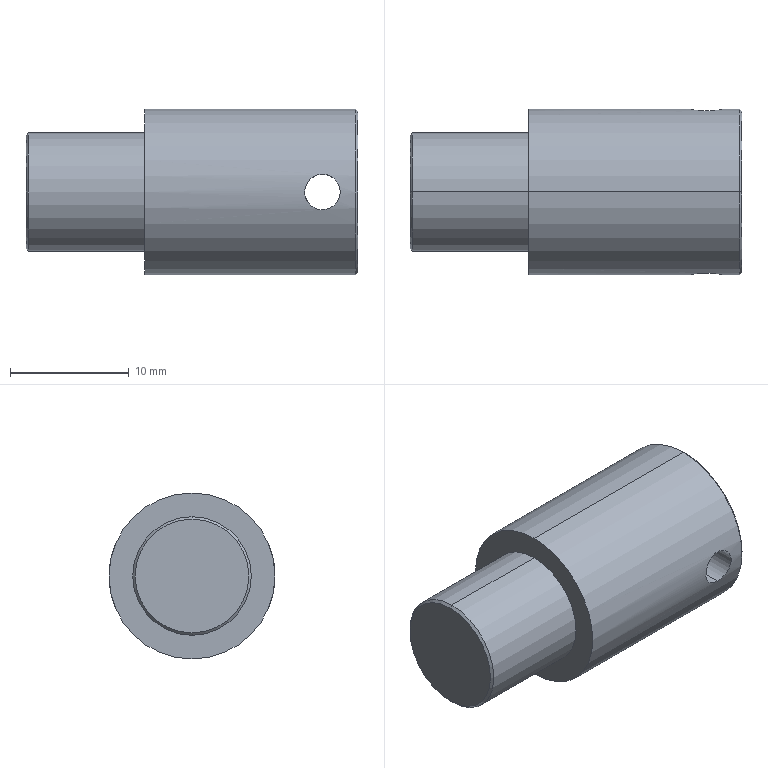Part | SolidWorks | features Chamfer 2, ICE 2, Revolution 1 | 1 solid | 13 faces | box 28 x 14 x 14 mm | volume 3456 mm3 | cylinder 6 | cone 4 | plane 3 | commonest cylinder face diameters 3 x2 10 x2 14 x2
STEP:
#1=CARTESIAN_POINT('',(28.,0.,-6.8));
#2=VERTEX_POINT('',#1);
#3=CARTESIAN_POINT('',(28.,0.,6.8));
#4=VERTEX_POINT('',#3);
#5=CARTESIAN_POINT('',(28.,0.,0.));
#6=DIRECTION('',(1.,0.,0.));
#7=DIRECTION('',(0.,0.,1.));
#8=AXIS2_PLACEMENT_3D('',#5,#6,#7);
#9=CIRCLE('',#8,6.8);
#10=EDGE_CURVE('',#2,#4,#9,.T.);
#11=ORIENTED_EDGE('',*,*,#10,.F.);
#12=CARTESIAN_POINT('',(27.8,0.,-7.));
#13=VERTEX_POINT('',#12);
#14=CARTESIAN_POINT('',(27.8,0.,-7.));
#15=DIRECTION('',(-0.7071,0.,-0.7071));
#16=VECTOR('',#15,1000.);
#17=LINE('',#14,#16);
#18=EDGE_CURVE('',#2,#13,#17,.T.);
#19=ORIENTED_EDGE('',*,*,#18,.T.);
#20=CARTESIAN_POINT('',(27.8,0.,7.));
#21=VERTEX_POINT('',#20);
#22=CARTESIAN_POINT('',(27.8,0.,0.));
#23=DIRECTION('',(-1.,0.,0.));
#24=DIRECTION('',(0.,0.,1.));
#25=AXIS2_PLACEMENT_3D('',#22,#23,#24);
#26=CIRCLE('',#25,7.);
#27=EDGE_CURVE('',#21,#13,#26,.T.);
#28=ORIENTED_EDGE('',*,*,#27,.F.);
#29=CARTESIAN_POINT('',(27.8,0.,7.));
#30=DIRECTION('',(-0.7071,0.,0.7071));
#31=VECTOR('',#30,1000.);
#32=LINE('',#29,#31);
#33=EDGE_CURVE('',#4,#21,#32,.T.);
#34=ORIENTED_EDGE('',*,*,#33,.F.);
#35=EDGE_LOOP('',(#11,#19,#28,#34));
#36=FACE_OUTER_BOUND('',#35,.T.);
#37=CARTESIAN_POINT('',(27.8,0.,0.));
#38=DIRECTION('',(-1.,0.,0.));
#39=DIRECTION('',(0.,0.,1.));
#40=AXIS2_PLACEMENT_3D('',#37,#38,#39);
#41=CONICAL_SURFACE('',#40,7.,0.7854);
#42=ADVANCED_FACE('',(#36),#41,.T.);
#43=CARTESIAN_POINT('',(25.,-6.837,-1.5));
#44=VERTEX_POINT('',#43);
#45=CARTESIAN_POINT('',(25.,-6.837,1.5));
#46=VERTEX_POINT('',#45);
#47=CARTESIAN_POINT('',(25.,-6.837,-1.5));
#48=CARTESIAN_POINT('',(24.901,-6.837,-1.5));
#49=CARTESIAN_POINT('',(24.803,-6.84,-1.49));
#50=CARTESIAN_POINT('',(24.611,-6.848,-1.452));
#51=CARTESIAN_POINT('',(24.515,-6.854,-1.423));
#52=CARTESIAN_POINT('',(24.244,-6.877,-1.31));
#53=CARTESIAN_POINT('',(24.077,-6.898,-1.199));
#54=CARTESIAN_POINT('',(23.802,-6.94,-0.923));
#55=CARTESIAN_POINT('',(23.69,-6.961,-0.7561));
#56=CARTESIAN_POINT('',(23.54,-6.991,-0.3952));
#57=CARTESIAN_POINT('',(23.5,-7.,-0.1978));
#58=CARTESIAN_POINT('',(23.5,-7.,0.1003));
#59=CARTESIAN_POINT('',(23.51,-6.998,0.198));
#60=CARTESIAN_POINT('',(23.548,-6.99,0.3901));
#61=CARTESIAN_POINT('',(23.577,-6.984,0.4855));
#62=CARTESIAN_POINT('',(23.653,-6.969,0.667));
#63=CARTESIAN_POINT('',(23.699,-6.96,0.753));
#64=CARTESIAN_POINT('',(23.808,-6.94,0.9158));
#65=CARTESIAN_POINT('',(23.871,-6.93,0.9926));
#66=CARTESIAN_POINT('',(24.078,-6.898,1.199));
#67=CARTESIAN_POINT('',(24.245,-6.877,1.311));
#68=CARTESIAN_POINT('',(24.606,-6.846,1.46));
#69=CARTESIAN_POINT('',(24.804,-6.837,1.5));
#70=CARTESIAN_POINT('',(25.,-6.837,1.5));
#71=B_SPLINE_CURVE_WITH_KNOTS('',3,(#47,#48,#49,#50,#51,#52,#53,#54,#55,#56,#57,#58,#59,#60,#61,#62,#63,#64,#65,#66,#67,#68,#69,#70),.UNSPECIFIED.,.F.,.F.,(4,2,2,2,2,2,2,2,2,2,2,4),(0.007055,0.007349,0.007643,0.008231,0.008819,0.009406,0.0097,0.009994,0.01029,0.01058,0.01117,0.01176),.UNSPECIFIED.);
#72=EDGE_CURVE('',#44,#46,#71,.T.);
#73=ORIENTED_EDGE('',*,*,#72,.F.);
#74=CARTESIAN_POINT('',(25.,6.837,-1.5));
#75=VERTEX_POINT('',#74);
#76=CARTESIAN_POINT('',(25.,-7.,-1.5));
#77=DIRECTION('',(0.,1.,0.));
#78=VECTOR('',#77,1000.);
#79=LINE('',#76,#78);
#80=EDGE_CURVE('',#44,#75,#79,.T.);
#81=ORIENTED_EDGE('',*,*,#80,.T.);
#82=CARTESIAN_POINT('',(25.,6.837,1.5));
#83=VERTEX_POINT('',#82);
#84=CARTESIAN_POINT('',(25.,6.837,1.5));
#85=CARTESIAN_POINT('',(24.901,6.837,1.5));
#86=CARTESIAN_POINT('',(24.803,6.84,1.49));
#87=CARTESIAN_POINT('',(24.611,6.848,1.452));
#88=CARTESIAN_POINT('',(24.515,6.854,1.423));
#89=CARTESIAN_POINT('',(24.334,6.869,1.348));
#90=CARTESIAN_POINT('',(24.248,6.878,1.301));
#91=CARTESIAN_POINT('',(24.085,6.898,1.193));
#92=CARTESIAN_POINT('',(24.008,6.909,1.129));
#93=CARTESIAN_POINT('',(23.801,6.94,0.9225));
#94=CARTESIAN_POINT('',(23.69,6.961,0.7555));
#95=CARTESIAN_POINT('',(23.54,6.991,0.3947));
#96=CARTESIAN_POINT('',(23.5,7.,0.1969));
#97=CARTESIAN_POINT('',(23.5,7.,-0.09757));
#98=CARTESIAN_POINT('',(23.51,6.998,-0.1973));
#99=CARTESIAN_POINT('',(23.548,6.99,-0.3899));
#100=CARTESIAN_POINT('',(23.577,6.984,-0.4836));
#101=CARTESIAN_POINT('',(23.69,6.961,-0.7565));
#102=CARTESIAN_POINT('',(23.8,6.941,-0.9216));
#103=CARTESIAN_POINT('',(24.009,6.908,-1.13));
#104=CARTESIAN_POINT('',(24.085,6.898,-1.192));
#105=CARTESIAN_POINT('',(24.247,6.878,-1.301));
#106=CARTESIAN_POINT('',(24.335,6.869,-1.348));
#107=CARTESIAN_POINT('',(24.516,6.854,-1.423));
#108=CARTESIAN_POINT('',(24.609,6.848,-1.452));
#109=CARTESIAN_POINT('',(24.802,6.84,-1.49));
#110=CARTESIAN_POINT('',(24.902,6.837,-1.5));
#111=CARTESIAN_POINT('',(25.,6.837,-1.5));
#112=B_SPLINE_CURVE_WITH_KNOTS('',3,(#84,#85,#86,#87,#88,#89,#90,#91,#92,#93,#94,#95,#96,#97,#98,#99,#100,#101,#102,#103,#104,#105,#106,#107,#108,#109,#110,#111),.UNSPECIFIED.,.F.,.F.,(4,2,2,2,2,2,2,2,2,2,2,2,2,4),(0.,0.000294,0.0005879,0.0008819,0.001176,0.001764,0.002352,0.002646,0.00294,0.003527,0.003821,0.004115,0.004409,0.004703),.UNSPECIFIED.);
#113=EDGE_CURVE('',#83,#75,#112,.T.);
#114=ORIENTED_EDGE('',*,*,#113,.F.);
#115=CARTESIAN_POINT('',(25.,-7.,1.5));
#116=DIRECTION('',(0.,1.,0.));
#117=VECTOR('',#116,1000.);
#118=LINE('',#115,#117);
#119=EDGE_CURVE('',#46,#83,#118,.T.);
#120=ORIENTED_EDGE('',*,*,#119,.F.);
#121=EDGE_LOOP('',(#73,#81,#114,#120));
#122=FACE_OUTER_BOUND('',#121,.T.);
#123=CARTESIAN_POINT('',(25.,-7.,0.));
#124=DIRECTION('',(0.,1.,0.));
#125=DIRECTION('',(0.,0.,1.));
#126=AXIS2_PLACEMENT_3D('',#123,#124,#125);
#127=CYLINDRICAL_SURFACE('',#126,1.5);
#128=ADVANCED_FACE('',(#122),#127,.F.);
#129=CARTESIAN_POINT('',(0.,0.,4.8));
#130=VERTEX_POINT('',#129);
#131=CARTESIAN_POINT('',(0.,0.,-4.8));
#132=VERTEX_POINT('',#131);
#133=CARTESIAN_POINT('',(0.,0.,0.));
#134=DIRECTION('',(-1.,0.,0.));
#135=DIRECTION('',(0.,0.,-1.));
#136=AXIS2_PLACEMENT_3D('',#133,#134,#135);
#137=CIRCLE('',#136,4.8);
#138=EDGE_CURVE('',#130,#132,#137,.T.);
#139=ORIENTED_EDGE('',*,*,#138,.F.);
#140=CARTESIAN_POINT('',(0.2,0.,5.));
#141=VERTEX_POINT('',#140);
#142=CARTESIAN_POINT('',(0.,0.,4.8));
#143=DIRECTION('',(0.7071,0.,0.7071));
#144=VECTOR('',#143,1000.);
#145=LINE('',#142,#144);
#146=EDGE_CURVE('',#130,#141,#145,.T.);
#147=ORIENTED_EDGE('',*,*,#146,.T.);
#148=CARTESIAN_POINT('',(0.2,0.,-5.));
#149=VERTEX_POINT('',#148);
#150=CARTESIAN_POINT('',(0.2,0.,0.));
#151=DIRECTION('',(1.,0.,0.));
#152=DIRECTION('',(0.,0.,-1.));
#153=AXIS2_PLACEMENT_3D('',#150,#151,#152);
#154=CIRCLE('',#153,5.);
#155=EDGE_CURVE('',#149,#141,#154,.T.);
#156=ORIENTED_EDGE('',*,*,#155,.F.);
#157=CARTESIAN_POINT('',(0.,0.,-4.8));
#158=DIRECTION('',(0.7071,0.,-0.7071));
#159=VECTOR('',#158,1000.);
#160=LINE('',#157,#159);
#161=EDGE_CURVE('',#132,#149,#160,.T.);
#162=ORIENTED_EDGE('',*,*,#161,.F.);
#163=EDGE_LOOP('',(#139,#147,#156,#162));
#164=FACE_OUTER_BOUND('',#163,.T.);
#165=CARTESIAN_POINT('',(0.,0.,0.));
#166=DIRECTION('',(1.,0.,0.));
#167=DIRECTION('',(0.,0.,-1.));
#168=AXIS2_PLACEMENT_3D('',#165,#166,#167);
#169=CONICAL_SURFACE('',#168,4.8,0.7854);
#170=ADVANCED_FACE('',(#164),#169,.T.);
#171=ORIENTED_EDGE('',*,*,#113,.T.);
#172=CARTESIAN_POINT('',(25.,6.837,-1.5));
#173=CARTESIAN_POINT('',(25.196,6.837,-1.5));
#174=CARTESIAN_POINT('',(25.394,6.846,-1.46));
#175=CARTESIAN_POINT('',(25.755,6.877,-1.311));
#176=CARTESIAN_POINT('',(25.922,6.898,-1.199));
#177=CARTESIAN_POINT('',(26.129,6.93,-0.9922));
#178=CARTESIAN_POINT('',(26.192,6.94,-0.9153));
#179=CARTESIAN_POINT('',(26.301,6.96,-0.753));
#180=CARTESIAN_POINT('',(26.347,6.969,-0.667));
#181=CARTESIAN_POINT('',(26.461,6.991,-0.3938));
#182=CARTESIAN_POINT('',(26.5,7.,-0.1987));
#183=CARTESIAN_POINT('',(26.5,7.,0.09833));
#184=CARTESIAN_POINT('',(26.49,6.998,0.1959));
#185=CARTESIAN_POINT('',(26.452,6.99,0.3882));
#186=CARTESIAN_POINT('',(26.423,6.984,0.4839));
#187=CARTESIAN_POINT('',(26.311,6.961,0.7556));
#188=CARTESIAN_POINT('',(26.199,6.94,0.9222));
#189=CARTESIAN_POINT('',(25.924,6.898,1.198));
#190=CARTESIAN_POINT('',(25.757,6.877,1.31));
#191=CARTESIAN_POINT('',(25.396,6.846,1.46));
#192=CARTESIAN_POINT('',(25.199,6.837,1.5));
#193=CARTESIAN_POINT('',(25.,6.837,1.5));
#194=B_SPLINE_CURVE_WITH_KNOTS('',3,(#172,#173,#174,#175,#176,#177,#178,#179,#180,#181,#182,#183,#184,#185,#186,#187,#188,#189,#190,#191,#192,#193),.UNSPECIFIED.,.F.,.F.,(4,2,2,2,2,2,2,2,2,2,4),(0.004703,0.005291,0.005879,0.006173,0.006467,0.007054,0.007348,0.007642,0.00823,0.008818,0.009405),.UNSPECIFIED.);
#195=EDGE_CURVE('',#75,#83,#194,.T.);
#196=ORIENTED_EDGE('',*,*,#195,.T.);
#197=EDGE_LOOP('',(#171,#196));
#198=FACE_BOUND('',#197,.T.);
#199=ORIENTED_EDGE('',*,*,#27,.T.);
#200=CARTESIAN_POINT('',(10.,0.,-7.));
#201=VERTEX_POINT('',#200);
#202=CARTESIAN_POINT('',(0.,0.,-7.));
#203=DIRECTION('',(-1.,0.,0.));
#204=VECTOR('',#203,1000.);
#205=LINE('',#202,#204);
#206=EDGE_CURVE('',#13,#201,#205,.T.);
#207=ORIENTED_EDGE('',*,*,#206,.T.);
#208=CARTESIAN_POINT('',(10.,0.,7.));
#209=VERTEX_POINT('',#208);
#210=CARTESIAN_POINT('',(10.,0.,0.));
#211=DIRECTION('',(-1.,0.,0.));
#212=DIRECTION('',(0.,0.,1.));
#213=AXIS2_PLACEMENT_3D('',#210,#211,#212);
#214=CIRCLE('',#213,7.);
#215=EDGE_CURVE('',#209,#201,#214,.T.);
#216=ORIENTED_EDGE('',*,*,#215,.F.);
#217=CARTESIAN_POINT('',(0.,0.,7.));
#218=DIRECTION('',(-1.,0.,0.));
#219=VECTOR('',#218,1000.);
#220=LINE('',#217,#219);
#221=EDGE_CURVE('',#21,#209,#220,.T.);
#222=ORIENTED_EDGE('',*,*,#221,.F.);
#223=EDGE_LOOP('',(#199,#207,#216,#222));
#224=FACE_OUTER_BOUND('',#223,.T.);
#225=CARTESIAN_POINT('',(0.,0.,0.));
#226=DIRECTION('',(-1.,0.,0.));
#227=DIRECTION('',(0.,0.,1.));
#228=AXIS2_PLACEMENT_3D('',#225,#226,#227);
#229=CYLINDRICAL_SURFACE('',#228,7.);
#230=ADVANCED_FACE('',(#198,#224),#229,.T.);
#231=CARTESIAN_POINT('',(10.,0.,5.));
#232=VERTEX_POINT('',#231);
#233=CARTESIAN_POINT('',(10.,0.,-5.));
#234=VERTEX_POINT('',#233);
#235=CARTESIAN_POINT('',(10.,0.,0.));
#236=DIRECTION('',(-1.,0.,0.));
#237=DIRECTION('',(0.,0.,1.));
#238=AXIS2_PLACEMENT_3D('',#235,#236,#237);
#239=CIRCLE('',#238,5.);
#240=EDGE_CURVE('',#232,#234,#239,.T.);
#241=ORIENTED_EDGE('',*,*,#240,.T.);
#242=CARTESIAN_POINT('',(0.,0.,-5.));
#243=DIRECTION('',(-1.,0.,0.));
#244=VECTOR('',#243,1000.);
#245=LINE('',#242,#244);
#246=EDGE_CURVE('',#234,#149,#245,.T.);
#247=ORIENTED_EDGE('',*,*,#246,.T.);
#248=ORIENTED_EDGE('',*,*,#155,.T.);
#249=CARTESIAN_POINT('',(0.,0.,5.));
#250=DIRECTION('',(-1.,0.,0.));
#251=VECTOR('',#250,1000.);
#252=LINE('',#249,#251);
#253=EDGE_CURVE('',#232,#141,#252,.T.);
#254=ORIENTED_EDGE('',*,*,#253,.F.);
#255=EDGE_LOOP('',(#241,#247,#248,#254));
#256=FACE_OUTER_BOUND('',#255,.T.);
#257=CARTESIAN_POINT('',(0.,0.,0.));
#258=DIRECTION('',(-1.,0.,0.));
#259=DIRECTION('',(0.,0.,1.));
#260=AXIS2_PLACEMENT_3D('',#257,#258,#259);
#261=CYLINDRICAL_SURFACE('',#260,5.);
#262=ADVANCED_FACE('',(#256),#261,.T.);
#263=CARTESIAN_POINT('',(0.,0.,0.));
#264=DIRECTION('',(-1.,0.,0.));
#265=DIRECTION('',(0.,0.,-1.));
#266=AXIS2_PLACEMENT_3D('',#263,#264,#265);
#267=CIRCLE('',#266,4.8);
#268=EDGE_CURVE('',#132,#130,#267,.T.);
#269=ORIENTED_EDGE('',*,*,#268,.T.);
#270=ORIENTED_EDGE('',*,*,#138,.T.);
#271=EDGE_LOOP('',(#269,#270));
#272=FACE_OUTER_BOUND('',#271,.T.);
#273=CARTESIAN_POINT('',(0.,0.,0.));
#274=DIRECTION('',(1.,0.,0.));
#275=DIRECTION('',(0.,0.,-1.));
#276=AXIS2_PLACEMENT_3D('',#273,#274,#275);
#277=PLANE('',#276);
#278=ADVANCED_FACE('',(#272),#277,.F.);
#279=ORIENTED_EDGE('',*,*,#246,.F.);
#280=CARTESIAN_POINT('',(10.,0.,0.));
#281=DIRECTION('',(-1.,0.,0.));
#282=DIRECTION('',(0.,0.,1.));
#283=AXIS2_PLACEMENT_3D('',#280,#281,#282);
#284=CIRCLE('',#283,5.);
#285=EDGE_CURVE('',#234,#232,#284,.T.);
#286=ORIENTED_EDGE('',*,*,#285,.T.);
#287=ORIENTED_EDGE('',*,*,#253,.T.);
#288=CARTESIAN_POINT('',(0.2,0.,0.));
#289=DIRECTION('',(1.,0.,0.));
#290=DIRECTION('',(0.,0.,-1.));
#291=AXIS2_PLACEMENT_3D('',#288,#289,#290);
#292=CIRCLE('',#291,5.);
#293=EDGE_CURVE('',#141,#149,#292,.T.);
#294=ORIENTED_EDGE('',*,*,#293,.T.);
#295=EDGE_LOOP('',(#279,#286,#287,#294));
#296=FACE_OUTER_BOUND('',#295,.T.);
#297=CARTESIAN_POINT('',(0.,0.,0.));
#298=DIRECTION('',(-1.,0.,0.));
#299=DIRECTION('',(0.,0.,1.));
#300=AXIS2_PLACEMENT_3D('',#297,#298,#299);
#301=CYLINDRICAL_SURFACE('',#300,5.);
#302=ADVANCED_FACE('',(#296),#301,.T.);
#303=ORIENTED_EDGE('',*,*,#240,.F.);
#304=ORIENTED_EDGE('',*,*,#285,.F.);
#305=EDGE_LOOP('',(#303,#304));
#306=FACE_BOUND('',#305,.T.);
#307=ORIENTED_EDGE('',*,*,#215,.T.);
#308=CARTESIAN_POINT('',(10.,0.,0.));
#309=DIRECTION('',(-1.,0.,0.));
#310=DIRECTION('',(0.,0.,1.));
#311=AXIS2_PLACEMENT_3D('',#308,#309,#310);
#312=CIRCLE('',#311,7.);
#313=EDGE_CURVE('',#201,#209,#312,.T.);
#314=ORIENTED_EDGE('',*,*,#313,.T.);
#315=EDGE_LOOP('',(#307,#314));
#316=FACE_OUTER_BOUND('',#315,.T.);
#317=CARTESIAN_POINT('',(10.,5.,0.));
#318=DIRECTION('',(1.,0.,0.));
#319=DIRECTION('',(0.,0.,-1.));
#320=AXIS2_PLACEMENT_3D('',#317,#318,#319);
#321=PLANE('',#320);
#322=ADVANCED_FACE('',(#306,#316),#321,.F.);
#323=ORIENTED_EDGE('',*,*,#206,.F.);
#324=CARTESIAN_POINT('',(27.8,0.,0.));
#325=DIRECTION('',(-1.,0.,0.));
#326=DIRECTION('',(0.,0.,1.));
#327=AXIS2_PLACEMENT_3D('',#324,#325,#326);
#328=CIRCLE('',#327,7.);
#329=EDGE_CURVE('',#13,#21,#328,.T.);
#330=ORIENTED_EDGE('',*,*,#329,.T.);
#331=ORIENTED_EDGE('',*,*,#221,.T.);
#332=ORIENTED_EDGE('',*,*,#313,.F.);
#333=EDGE_LOOP('',(#323,#330,#331,#332));
#334=FACE_OUTER_BOUND('',#333,.T.);
#335=CARTESIAN_POINT('',(25.,-6.837,1.5));
#336=CARTESIAN_POINT('',(25.098,-6.837,1.5));
#337=CARTESIAN_POINT('',(25.198,-6.84,1.49));
#338=CARTESIAN_POINT('',(25.39,-6.848,1.452));
#339=CARTESIAN_POINT('',(25.484,-6.854,1.423));
#340=CARTESIAN_POINT('',(25.757,-6.877,1.31));
#341=CARTESIAN_POINT('',(25.922,-6.898,1.2));
#342=CARTESIAN_POINT('',(26.131,-6.93,0.9905));
#343=CARTESIAN_POINT('',(26.193,-6.94,0.9151));
#344=CARTESIAN_POINT('',(26.301,-6.96,0.7528));
#345=CARTESIAN_POINT('',(26.348,-6.969,0.665));
#346=CARTESIAN_POINT('',(26.423,-6.984,0.4837));
#347=CARTESIAN_POINT('',(26.452,-6.99,0.3902));
#348=CARTESIAN_POINT('',(26.49,-6.998,0.1973));
#349=CARTESIAN_POINT('',(26.5,-7.,0.09772));
#350=CARTESIAN_POINT('',(26.5,-7.,-0.1964));
#351=CARTESIAN_POINT('',(26.46,-6.991,-0.3943));
#352=CARTESIAN_POINT('',(26.31,-6.961,-0.7555));
#353=CARTESIAN_POINT('',(26.199,-6.94,-0.9221));
#354=CARTESIAN_POINT('',(25.992,-6.909,-1.13));
#355=CARTESIAN_POINT('',(25.915,-6.898,-1.193));
#356=CARTESIAN_POINT('',(25.752,-6.878,-1.301));
#357=CARTESIAN_POINT('',(25.666,-6.869,-1.347));
#358=CARTESIAN_POINT('',(25.393,-6.846,-1.461));
#359=CARTESIAN_POINT('',(25.198,-6.837,-1.5));
#360=CARTESIAN_POINT('',(25.,-6.837,-1.5));
#361=B_SPLINE_CURVE_WITH_KNOTS('',3,(#335,#336,#337,#338,#339,#340,#341,#342,#343,#344,#345,#346,#347,#348,#349,#350,#351,#352,#353,#354,#355,#356,#357,#358,#359,#360),.UNSPECIFIED.,.F.,.F.,(4,2,2,2,2,2,2,2,2,2,2,2,4),(0.002352,0.002646,0.00294,0.003528,0.003822,0.004116,0.00441,0.004704,0.005292,0.005879,0.006173,0.006467,0.007055),.UNSPECIFIED.);
#362=EDGE_CURVE('',#46,#44,#361,.T.);
#363=ORIENTED_EDGE('',*,*,#362,.T.);
#364=ORIENTED_EDGE('',*,*,#72,.T.);
#365=EDGE_LOOP('',(#363,#364));
#366=FACE_BOUND('',#365,.T.);
#367=CARTESIAN_POINT('',(0.,0.,0.));
#368=DIRECTION('',(-1.,0.,0.));
#369=DIRECTION('',(0.,0.,1.));
#370=AXIS2_PLACEMENT_3D('',#367,#368,#369);
#371=CYLINDRICAL_SURFACE('',#370,7.);
#372=ADVANCED_FACE('',(#334,#366),#371,.T.);
#373=CARTESIAN_POINT('',(28.,0.,0.));
#374=DIRECTION('',(1.,0.,0.));
#375=DIRECTION('',(0.,0.,1.));
#376=AXIS2_PLACEMENT_3D('',#373,#374,#375);
#377=CIRCLE('',#376,6.8);
#378=EDGE_CURVE('',#4,#2,#377,.T.);
#379=ORIENTED_EDGE('',*,*,#378,.T.);
#380=ORIENTED_EDGE('',*,*,#10,.T.);
#381=EDGE_LOOP('',(#379,#380));
#382=FACE_OUTER_BOUND('',#381,.T.);
#383=CARTESIAN_POINT('',(28.,7.,0.));
#384=DIRECTION('',(-1.,0.,0.));
#385=DIRECTION('',(0.,0.,1.));
#386=AXIS2_PLACEMENT_3D('',#383,#384,#385);
#387=PLANE('',#386);
#388=ADVANCED_FACE('',(#382),#387,.F.);
#389=ORIENTED_EDGE('',*,*,#146,.F.);
#390=ORIENTED_EDGE('',*,*,#268,.F.);
#391=ORIENTED_EDGE('',*,*,#161,.T.);
#392=ORIENTED_EDGE('',*,*,#293,.F.);
#393=EDGE_LOOP('',(#389,#390,#391,#392));
#394=FACE_OUTER_BOUND('',#393,.T.);
#395=CARTESIAN_POINT('',(0.,0.,0.));
#396=DIRECTION('',(1.,0.,0.));
#397=DIRECTION('',(0.,0.,-1.));
#398=AXIS2_PLACEMENT_3D('',#395,#396,#397);
#399=CONICAL_SURFACE('',#398,4.8,0.7854);
#400=ADVANCED_FACE('',(#394),#399,.T.);
#401=ORIENTED_EDGE('',*,*,#80,.F.);
#402=ORIENTED_EDGE('',*,*,#362,.F.);
#403=ORIENTED_EDGE('',*,*,#119,.T.);
#404=ORIENTED_EDGE('',*,*,#195,.F.);
#405=EDGE_LOOP('',(#401,#402,#403,#404));
#406=FACE_OUTER_BOUND('',#405,.T.);
#407=CARTESIAN_POINT('',(25.,-7.,0.));
#408=DIRECTION('',(0.,1.,0.));
#409=DIRECTION('',(0.,0.,1.));
#410=AXIS2_PLACEMENT_3D('',#407,#408,#409);
#411=CYLINDRICAL_SURFACE('',#410,1.5);
#412=ADVANCED_FACE('',(#406),#411,.F.);
#413=ORIENTED_EDGE('',*,*,#18,.F.);
#414=ORIENTED_EDGE('',*,*,#378,.F.);
#415=ORIENTED_EDGE('',*,*,#33,.T.);
#416=ORIENTED_EDGE('',*,*,#329,.F.);
#417=EDGE_LOOP('',(#413,#414,#415,#416));
#418=FACE_OUTER_BOUND('',#417,.T.);
#419=CARTESIAN_POINT('',(27.8,0.,0.));
#420=DIRECTION('',(-1.,0.,0.));
#421=DIRECTION('',(0.,0.,1.));
#422=AXIS2_PLACEMENT_3D('',#419,#420,#421);
#423=CONICAL_SURFACE('',#422,7.,0.7854);
#424=ADVANCED_FACE('',(#418),#423,.T.);
#425=CLOSED_SHELL('',(#42,#128,#170,#230,#262,#278,#302,#322,#372,#388,#400,#412,#424));
#426=MANIFOLD_SOLID_BREP('',#425);
#427=CARTESIAN_POINT('',(0.,0.,0.));
#428=DIRECTION('',(0.,0.,1.));
#429=DIRECTION('',(1.,0.,0.));
#430=AXIS2_PLACEMENT_3D('',#427,#428,#429);
#431=(LENGTH_UNIT()NAMED_UNIT(*)SI_UNIT(.MILLI.,.METRE.));
#432=UNCERTAINTY_MEASURE_WITH_UNIT(LENGTH_MEASURE(0.00001),#431,'','');
#433=(NAMED_UNIT(*)PLANE_ANGLE_UNIT()SI_UNIT($,.RADIAN.));
#434=(NAMED_UNIT(*)SI_UNIT($,.STERADIAN.)SOLID_ANGLE_UNIT());
#435=(GEOMETRIC_REPRESENTATION_CONTEXT(3)GLOBAL_UNCERTAINTY_ASSIGNED_CONTEXT((#432))GLOBAL_UNIT_ASSIGNED_CONTEXT((#431,#433,#434))REPRESENTATION_CONTEXT('',''));
#436=ADVANCED_BREP_SHAPE_REPRESENTATION('',(#426,#430),#435);